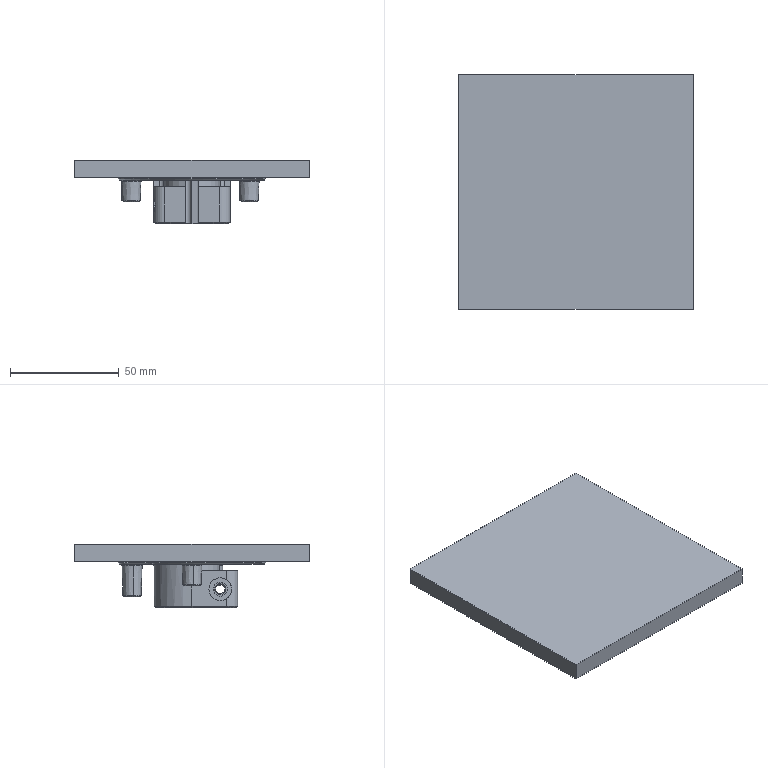NC program | NX | posted with a generic post | part box 108 x 108 x 29 mm
Lines 3489 to 4515 of 23883:
(CAVITY_MILL_COPY_COPY , TOOL : D4)
N6958 T15 M6
N6960 G54
N6962 G17 G0 G90 X0. Y-7.141 S9500 M3
N6964 G43 Z30. H15
N6966 Z-0.385
N6968 G94 G1 X0.5 Y-9.933 F1000.
N6970 G3 X1. Y-9.067 R1.
N6972 G1 X0.541 F1400.
N6974 X0.513 Y-9.112
N6976 X0.51 Y-9.166
N6978 G2 X-0.51 Y-9.166 R0.52
N6980 G1 X-0.513 Y-9.112
N6982 X-0.541 Y-9.067
N6984 X-1.
N6986 Y-20.799
N6988 G3 X-0.51 Y-20.398 R0.5
N6990 G2 X0.51 Y-20.398 R0.52
N6992 G3 X1. Y-20.799 R0.5
N6994 G1 Y-9.067
N6996 G3 X0.5 Y-8.201 R1.
N6998 G1 X0.447 Y-7.069
N7000 G0 X0. Y-7.141 Z-0.769
N7002 G1 X0.5 Y-9.933 F1000.
N7004 G3 X1. Y-9.067 R1.
N7006 G1 X0.541 F1400.
N7008 X0.513 Y-9.112
N7010 X0.51 Y-9.166
N7012 G2 X-0.51 Y-9.166 R0.52
N7014 G1 X-0.513 Y-9.112
N7016 X-0.541 Y-9.067
N7018 X-1.
N7020 Y-20.799
N7022 G3 X-0.51 Y-20.398 R0.5
N7024 G2 X0.51 Y-20.398 R0.52
N7026 G3 X1. Y-20.799 R0.5
N7028 G1 Y-9.067
N7030 G3 X0.5 Y-8.201 R1.
N7032 G1 X0.447 Y-7.069
N7034 G0 X0. Y-7.141 Z-1.154
N7036 G1 X0.5 Y-9.933 F1000.
N7038 G3 X1. Y-9.067 R1.
N7040 G1 X0.541 F1400.
N7042 X0.513 Y-9.112
N7044 X0.51 Y-9.166
N7046 G2 X-0.51 Y-9.166 R0.52
N7048 G1 X-0.513 Y-9.112
N7050 X-0.541 Y-9.067
N7052 X-1.
N7054 Y-20.799
N7056 G3 X-0.51 Y-20.398 R0.5
N7058 G2 X0.51 Y-20.398 R0.52
N7060 G3 X1. Y-20.799 R0.5
N7062 G1 Y-9.067
N7064 G3 X0.5 Y-8.201 R1.
N7066 G1 X0.447 Y-7.069
N7068 G0 X0. Y-7.141 Z-1.538
N7070 G1 X0.5 Y-9.933 F1000.
N7072 G3 X1. Y-9.067 R1.
N7074 G1 X0.541 F1400.
N7076 X0.513 Y-9.112
N7078 X0.51 Y-9.166
N7080 G2 X-0.51 Y-9.166 R0.52
N7082 G1 X-0.513 Y-9.112
N7084 X-0.541 Y-9.067
N7086 X-1.
N7088 Y-20.799
N7090 G3 X-0.51 Y-20.398 R0.5
N7092 G2 X0.51 Y-20.398 R0.52
N7094 G3 X1. Y-20.799 R0.5
N7096 G1 Y-9.067
N7098 G3 X0.5 Y-8.201 R1.
N7100 G1 X0.447 Y-7.069
N7102 G0 X0. Y-7.141 Z-1.923
N7104 G1 X0.5 Y-9.933 F1000.
N7106 G3 X1. Y-9.067 R1.
N7108 G1 X0.541 F1400.
N7110 X0.513 Y-9.112
N7112 X0.51 Y-9.166
N7114 G2 X-0.51 Y-9.166 R0.52
N7116 G1 X-0.513 Y-9.112
N7118 X-0.541 Y-9.067
N7120 X-1.
N7122 Y-20.799
N7124 G3 X-0.51 Y-20.398 R0.5
N7126 G2 X0.51 Y-20.398 R0.52
N7128 G3 X1. Y-20.799 R0.5
N7130 G1 Y-9.067
N7132 G3 X0.5 Y-8.201 R1.
N7134 G1 X0.447 Y-7.069
N7136 G0 X0. Y-7.141 Z-2.308
N7138 G1 X0.5 Y-9.933 F1000.
N7140 G3 X1. Y-9.067 R1.
N7142 G1 X0.541 F1400.
N7144 X0.513 Y-9.112
N7146 X0.51 Y-9.166
N7148 G2 X-0.51 Y-9.166 R0.52
N7150 G1 X-0.513 Y-9.112
N7152 X-0.541 Y-9.067
N7154 X-1.
N7156 Y-20.799
N7158 G3 X-0.51 Y-20.398 R0.5
N7160 G2 X0.51 Y-20.398 R0.52
N7162 G3 X1. Y-20.799 R0.5
N7164 G1 Y-9.067
N7166 G3 X0.5 Y-8.201 R1.
N7168 G1 X0.447 Y-7.069
N7170 G0 X0. Y-7.141 Z-2.692
N7172 G1 X0.5 Y-9.933 F1000.
N7174 G3 X1. Y-9.067 R1.
N7176 G1 X0.541 F1400.
N7178 X0.513 Y-9.112
N7180 X0.51 Y-9.166
N7182 G2 X-0.51 Y-9.166 R0.52
N7184 G1 X-0.513 Y-9.112
N7186 X-0.541 Y-9.067
N7188 X-1.
N7190 Y-20.799
N7192 G3 X-0.51 Y-20.398 R0.5
N7194 G2 X0.51 Y-20.398 R0.52
N7196 G3 X1. Y-20.799 R0.5
N7198 G1 Y-9.067
N7200 G3 X0.5 Y-8.201 R1.
N7202 G1 X0.447 Y-7.069
N7204 G0 X0. Y-7.141 Z-3.077
N7206 G1 X0.5 Y-9.933 F1000.
N7208 G3 X1. Y-9.067 R1.
N7210 G1 X0.541 F1400.
N7212 X0.513 Y-9.112
N7214 X0.51 Y-9.166
N7216 G2 X-0.51 Y-9.166 R0.52
N7218 G1 X-0.513 Y-9.112
N7220 X-0.541 Y-9.067
N7222 X-1.
N7224 Y-20.799
N7226 G3 X-0.51 Y-20.398 R0.5
N7228 G2 X0.51 Y-20.398 R0.52
N7230 G3 X1. Y-20.799 R0.5
N7232 G1 Y-9.067
N7234 G3 X0.5 Y-8.201 R1.
N7236 G1 X0.447 Y-7.069
N7238 G0 X0. Y-7.141 Z-3.462
N7240 G1 X0.5 Y-9.933 F1000.
N7242 G3 X1. Y-9.067 R1.
N7244 G1 X0.541 F1400.
N7246 X0.513 Y-9.112
N7248 X0.51 Y-9.166
N7250 G2 X-0.51 Y-9.166 R0.52
N7252 G1 X-0.513 Y-9.112
N7254 X-0.541 Y-9.067
N7256 X-1.
N7258 Y-20.799
N7260 G3 X-0.51 Y-20.398 R0.5
N7262 G2 X0.51 Y-20.398 R0.52
N7264 G3 X1. Y-20.799 R0.5
N7266 G1 Y-9.067
N7268 G3 X0.5 Y-8.201 R1.
N7270 G1 X0.447 Y-7.069
N7272 G0 X0. Y-7.141 Z-3.846
N7274 G1 X0.5 Y-9.933 F1000.
N7276 G3 X1. Y-9.067 R1.
N7278 G1 X0.541 F1400.
N7280 X0.513 Y-9.112
N7282 X0.51 Y-9.166
N7284 G2 X-0.51 Y-9.166 R0.52
N7286 G1 X-0.513 Y-9.112
N7288 X-0.541 Y-9.067
N7290 X-1.
N7292 Y-20.799
N7294 G3 X-0.51 Y-20.398 R0.5
N7296 G2 X0.51 Y-20.398 R0.52
N7298 G3 X1. Y-20.799 R0.5
N7300 G1 Y-9.067
N7302 G3 X0.5 Y-8.201 R1.
N7304 G1 X0.447 Y-7.069
N7306 G0 X0. Y-7.141 Z-4.231
N7308 G1 X0.5 Y-9.933 F1000.
N7310 G3 X1. Y-9.067 R1.
N7312 G1 X0.541 F1400.
N7314 X0.513 Y-9.112
N7316 X0.51 Y-9.166
N7318 G2 X-0.51 Y-9.166 R0.52
N7320 G1 X-0.513 Y-9.112
N7322 X-0.541 Y-9.067
N7324 X-1.
N7326 Y-20.8
N7328 G3 X-0.51 Y-20.398 R0.5
N7330 G2 X0.51 Y-20.398 R0.52
N7332 G3 X1. Y-20.8 R0.5
N7334 G1 Y-9.067
N7336 G3 X0.5 Y-8.201 R1.
N7338 G1 X0.447 Y-7.069
N7340 G0 X0. Y-7.141 Z-4.615
N7342 G1 X0.5 Y-9.933 F1000.
N7344 G3 X1. Y-9.067 R1.
N7346 G1 X0.541 F1400.
N7348 X0.513 Y-9.112
N7350 X0.51 Y-9.166
N7352 G2 X-0.51 Y-9.166 R0.52
N7354 G1 X-0.513 Y-9.112
N7356 X-0.541 Y-9.067
N7358 X-1.
N7360 Y-20.8
N7362 G3 X-0.51 Y-20.398 R0.5
N7364 G2 X0.51 Y-20.398 R0.52
N7366 G3 X1. Y-20.8 R0.5
N7368 G1 Y-9.067
N7370 G3 X0.5 Y-8.201 R1.
N7372 G1 X0.447 Y-7.069
N7374 G0 X0. Y-7.141 Z-5.
N7376 G1 X0.5 Y-9.933 F1000.
N7378 G3 X1. Y-9.067 R1.
N7380 G1 X0.541 F1400.
N7382 X0.513 Y-9.112
N7384 X0.51 Y-9.166
N7386 G2 X-0.51 Y-9.166 R0.52
N7388 G1 X-0.513 Y-9.112
N7390 X-0.541 Y-9.067
N7392 X-1.
N7394 Y-20.8
N7396 G3 X-0.51 Y-20.398 R0.5
N7398 G2 X0.51 Y-20.398 R0.52
N7400 G3 X1. Y-20.8 R0.5
N7402 G1 Y-9.067
N7404 G3 X0.5 Y-8.201 R1.
N7406 G1 X0.447 Y-7.069
N7408 G0 X0. Y-7.141 Z-5.385
N7410 G1 X0.5 Y-9.933 F1000.
N7412 G3 X1. Y-9.067 R1.
N7414 G1 X0.541 F1400.
N7416 X0.513 Y-9.112
N7418 X0.51 Y-9.166
N7420 G2 X-0.51 Y-9.166 R0.52
N7422 G1 X-0.513 Y-9.112
N7424 X-0.541 Y-9.067
N7426 X-1.
N7428 Y-20.8
N7430 G3 X-0.51 Y-20.398 R0.5
N7432 G2 X0.51 Y-20.398 R0.52
N7434 G3 X1. Y-20.8 R0.5
N7436 G1 Y-9.067
N7438 G3 X0.5 Y-8.201 R1.
N7440 G1 X0.447 Y-7.069
N7442 G0 X0. Y-7.141 Z-5.769
N7444 G1 X0.5 Y-9.933 F1000.
N7446 G3 X1. Y-9.067 R1.
N7448 G1 X0.541 F1400.
N7450 X0.513 Y-9.112
N7452 X0.51 Y-9.166
N7454 G2 X-0.51 Y-9.166 R0.52
N7456 G1 X-0.513 Y-9.112
N7458 X-0.541 Y-9.067
N7460 X-1.
N7462 Y-20.8
N7464 G3 X-0.51 Y-20.398 R0.5
N7466 G2 X0.51 Y-20.398 R0.52
N7468 G3 X1. Y-20.8 R0.5
N7470 G1 Y-9.067
N7472 G3 X0.5 Y-8.201 R1.
N7474 G1 X0.447 Y-7.069
N7476 G0 X0. Y-7.141 Z-6.154
N7478 G1 X0.5 Y-9.933 F1000.
N7480 G3 X1. Y-9.067 R1.
N7482 G1 X0.542 F1400.
N7484 X0.514 Y-9.114
N7486 X0.51 Y-9.169
N7488 G2 X-0.51 Y-9.169 R0.52
N7490 G1 X-0.514 Y-9.114
N7492 X-0.542 Y-9.067
N7494 X-1.
N7496 Y-20.8
N7498 G3 X-0.51 Y-20.398 R0.5
N7500 G2 X0.51 Y-20.398 R0.52
N7502 G3 X1. Y-20.8 R0.5
N7504 G1 Y-9.067
N7506 G3 X0.5 Y-8.201 R1.
N7508 G1 X0.445 Y-7.069
N7510 G0 X0. Y-7.141 Z-6.538
N7512 G1 X0.5 Y-9.933 F1000.
N7514 G3 X1. Y-9.067 R1.
N7516 G1 X0.542 F1400.
N7518 X0.514 Y-9.114
N7520 X0.51 Y-9.169
N7522 G2 X-0.51 Y-9.169 R0.52
N7524 G1 X-0.514 Y-9.114
N7526 X-0.542 Y-9.067
N7528 X-1.
N7530 Y-20.8
N7532 G3 X-0.51 Y-20.398 R0.5
N7534 G2 X0.51 Y-20.398 R0.52
N7536 G3 X1. Y-20.8 R0.5
N7538 G1 Y-9.067
N7540 G3 X0.5 Y-8.201 R1.
N7542 G1 X0.445 Y-7.069
N7544 G0 X0. Y-7.141 Z-6.923
N7546 G1 X0.5 Y-9.933 F1000.
N7548 G3 X1. Y-9.067 R1.
N7550 G1 X0.542 F1400.
N7552 X0.514 Y-9.114
N7554 X0.51 Y-9.169
N7556 G2 X-0.51 Y-9.169 R0.52
N7558 G1 X-0.514 Y-9.114
N7560 X-0.542 Y-9.067
N7562 X-1.
N7564 Y-20.8
N7566 G3 X-0.51 Y-20.398 R0.5
N7568 G2 X0.51 Y-20.398 R0.52
N7570 G3 X1. Y-20.8 R0.5
N7572 G1 Y-9.067
N7574 G3 X0.5 Y-8.201 R1.
N7576 G1 X0.445 Y-7.069
N7578 G0 X0. Y-7.141 Z-7.308
N7580 G1 X0.5 Y-9.933 F1000.
N7582 G3 X1. Y-9.067 R1.
N7584 G1 X0.541 F1400.
N7586 X0.513 Y-9.112
N7588 X0.51 Y-9.166
N7590 G2 X-0.51 Y-9.166 R0.52
N7592 G1 X-0.513 Y-9.112
N7594 X-0.541 Y-9.067
N7596 X-1.
N7598 Y-20.8
N7600 G3 X-0.51 Y-20.398 R0.5
N7602 G2 X0.51 Y-20.398 R0.52
N7604 G3 X1. Y-20.8 R0.5
N7606 G1 Y-9.067
N7608 G3 X0.5 Y-8.201 R1.
N7610 G1 X0.447 Y-7.069
N7612 G0 X0. Y-7.141 Z-7.692
N7614 G1 X0.5 Y-9.933 F1000.
N7616 G3 X1. Y-9.067 R1.
N7618 G1 X0.541 F1400.
N7620 X0.513 Y-9.112
N7622 X0.51 Y-9.166
N7624 G2 X-0.51 Y-9.166 R0.52
N7626 G1 X-0.513 Y-9.112
N7628 X-0.541 Y-9.067
N7630 X-1.
N7632 Y-20.8
N7634 G3 X-0.51 Y-20.398 R0.5
N7636 G2 X0.51 Y-20.398 R0.52
N7638 G3 X1. Y-20.8 R0.5
N7640 G1 Y-9.067
N7642 G3 X0.5 Y-8.201 R1.
N7644 G1 X0.447 Y-7.069
N7646 G0 X0. Y-7.141 Z-8.077
N7648 G1 X0.5 Y-9.933 F1000.
N7650 G3 X1. Y-9.067 R1.
N7652 G1 X0.541 F1400.
N7654 X0.513 Y-9.112
N7656 X0.51 Y-9.166
N7658 G2 X-0.51 Y-9.166 R0.52
N7660 G1 X-0.513 Y-9.112
N7662 X-0.541 Y-9.067
N7664 X-1.
N7666 Y-20.8
N7668 G3 X-0.51 Y-20.398 R0.5
N7670 G2 X0.51 Y-20.398 R0.52
N7672 G3 X1. Y-20.8 R0.5
N7674 G1 Y-9.067
N7676 G3 X0.5 Y-8.201 R1.
N7678 G1 X0.447 Y-7.069
N7680 G0 X0. Y-7.141 Z-8.462
N7682 G1 X0.5 Y-9.933 F1000.
N7684 G3 X1. Y-9.067 R1.
N7686 G1 X0.541 F1400.
N7688 X0.513 Y-9.112
N7690 X0.51 Y-9.166
N7692 G2 X-0.51 Y-9.166 R0.52
N7694 G1 X-0.513 Y-9.112
N7696 X-0.541 Y-9.067
N7698 X-1.
N7700 Y-20.8
N7702 G3 X-0.51 Y-20.399 R0.5
N7704 G2 X0.51 Y-20.399 R0.52
N7706 G3 X1. Y-20.8 R0.5
N7708 G1 Y-9.067
N7710 G3 X0.5 Y-8.201 R1.
N7712 G1 X0.447 Y-7.069
N7714 G0 X0. Y-7.141 Z-8.846
N7716 G1 X0.5 Y-9.933 F1000.
N7718 G3 X1. Y-9.067 R1.
N7720 G1 X0.541 F1400.
N7722 X0.513 Y-9.112
N7724 X0.51 Y-9.166
N7726 G2 X-0.51 Y-9.166 R0.52
N7728 G1 X-0.513 Y-9.112
N7730 X-0.541 Y-9.067
N7732 X-1.
N7734 Y-20.8
N7736 G3 X-0.51 Y-20.399 R0.5
N7738 G2 X0.51 Y-20.399 R0.52
N7740 G3 X1. Y-20.8 R0.5
N7742 G1 Y-9.067
N7744 G3 X0.5 Y-8.201 R1.
N7746 G1 X0.447 Y-7.069
N7748 G0 X0. Y-7.141 Z-9.231
N7750 G1 X0.5 Y-9.933 F1000.
N7752 G3 X1. Y-9.067 R1.
N7754 G1 X0.541 F1400.
N7756 X0.513 Y-9.112
N7758 X0.51 Y-9.166
N7760 G2 X-0.51 Y-9.166 R0.52
N7762 G1 X-0.513 Y-9.112
N7764 X-0.541 Y-9.067
N7766 X-1.
N7768 Y-20.8
N7770 G3 X-0.51 Y-20.399 R0.5
N7772 G2 X0.51 Y-20.399 R0.52
N7774 G3 X1. Y-20.8 R0.5
N7776 G1 Y-9.067
N7778 G3 X0.5 Y-8.201 R1.
N7780 G1 X0.447 Y-7.069
N7782 G0 X0. Y-7.141 Z-9.615
N7784 G1 X0.5 Y-9.933 F1000.
N7786 G3 X1. Y-9.067 R1.
N7788 G1 X0.541 F1400.
N7790 X0.513 Y-9.112
N7792 X0.51 Y-9.166
N7794 G2 X-0.51 Y-9.166 R0.52
N7796 G1 X-0.513 Y-9.112
N7798 X-0.541 Y-9.067
N7800 X-1.
N7802 Y-20.8
N7804 G3 X-0.51 Y-20.399 R0.5
N7806 G2 X0.51 Y-20.399 R0.52
N7808 G3 X1. Y-20.8 R0.5
N7810 G1 Y-9.067
N7812 G3 X0.5 Y-8.201 R1.
N7814 G1 X0.447 Y-7.069
N7816 G0 X0. Y-7.141 Z-10.
N7818 G1 X0.5 Y-9.933 F1000.
N7820 G3 X1. Y-9.067 R1.
N7822 G1 X0.542 F1400.
N7824 X0.514 Y-9.114
N7826 X0.51 Y-9.169
N7828 G2 X-0.51 Y-9.169 R0.52
N7830 G1 X-0.514 Y-9.114
N7832 X-0.542 Y-9.067
N7834 X-1.
N7836 Y-20.8
N7838 G3 X-0.51 Y-20.399 R0.5
N7840 G2 X0.51 Y-20.399 R0.52
N7842 G3 X1. Y-20.8 R0.5
N7844 G1 Y-9.067
N7846 G3 X0.5 Y-8.201 R1.
N7848 G1 X0.445 Y-7.069
N7850 G0 X0. Y-7.141 Z-10.4
N7852 G1 X0.5 Y-9.933 F1000.
N7854 G3 X1. Y-9.067 R1.
N7856 G1 X0.542 F1400.
N7858 X0.514 Y-9.114
N7860 X0.51 Y-9.169
N7862 G2 X-0.51 Y-9.169 R0.52
N7864 G1 X-0.514 Y-9.114
N7866 X-0.542 Y-9.067
N7868 X-1.
N7870 Y-20.8
N7872 G3 X-0.51 Y-20.399 R0.5
N7874 G2 X0.51 Y-20.399 R0.52
N7876 G3 X1. Y-20.8 R0.5
N7878 G1 Y-9.067
N7880 G3 X0.5 Y-8.201 R1.
N7882 G1 X0.445 Y-7.069
N7884 G0 X0. Y-7.141 Z-10.8
N7886 G1 X0.5 Y-9.933 F1000.
N7888 G3 X1. Y-9.067 R1.
N7890 G1 X0.542 F1400.
N7892 X0.514 Y-9.114
N7894 X0.51 Y-9.169
N7896 G2 X-0.51 Y-9.169 R0.52
N7898 G1 X-0.514 Y-9.114
N7900 X-0.542 Y-9.067
N7902 X-1.
N7904 Y-20.8
N7906 G3 X-0.51 Y-20.399 R0.5
N7908 G2 X0.51 Y-20.399 R0.52
N7910 G3 X1. Y-20.8 R0.5
N7912 G1 Y-9.067
N7914 G3 X0.5 Y-8.201 R1.
N7916 G1 X0.445 Y-7.069
N7918 G0 X0. Y-7.141 Z-11.2
N7920 G1 X0.5 Y-9.933 F1000.
N7922 G3 X1. Y-9.067 R1.
N7924 G1 X0.542 F1400.
N7926 X0.514 Y-9.114
N7928 X0.51 Y-9.169
N7930 G2 X-0.51 Y-9.169 R0.52
N7932 G1 X-0.514 Y-9.114
N7934 X-0.542 Y-9.067
N7936 X-1.
N7938 Y-20.8
N7940 G3 X-0.51 Y-20.399 R0.5
N7942 G2 X0.51 Y-20.399 R0.52
N7944 G3 X1. Y-20.8 R0.5
N7946 G1 Y-9.067
N7948 G3 X0.5 Y-8.201 R1.
N7950 G1 X0.445 Y-7.069
N7952 G0 X0. Y-7.141 Z-11.6
N7954 G1 X0.5 Y-9.933 F1000.
N7956 G3 X1. Y-9.067 R1.
N7958 G1 X0.542 F1400.
N7960 X0.514 Y-9.114
N7962 X0.51 Y-9.169
N7964 G2 X-0.51 Y-9.169 R0.52
N7966 G1 X-0.514 Y-9.114
N7968 X-0.542 Y-9.067
N7970 X-1.
N7972 Y-20.8
N7974 G3 X-0.51 Y-20.399 R0.5
N7976 G2 X0.51 Y-20.399 R0.52
N7978 G3 X1. Y-20.8 R0.5
N7980 G1 Y-9.067
N7982 G3 X0.5 Y-8.201 R1.
N7984 G1 X0.445 Y-7.069
N7986 G0 X0. Y-7.141 Z-12.
N7988 G1 X0.5 Y-9.933 F1000.
N7990 G3 X1. Y-9.067 R1.
N7992 G1 X0.542 F1400.
N7994 X0.514 Y-9.114
N7996 X0.51 Y-9.168
N7998 G2 X-0.51 Y-9.168 R0.52
N8000 G1 X-0.514 Y-9.114
N8002 X-0.542 Y-9.067
N8004 X-1.
N8006 Y-20.8
N8008 G3 X-0.51 Y-20.399 R0.5
N8010 G2 X0.51 Y-20.399 R0.52
N8012 G3 X1. Y-20.8 R0.5
N8014 G1 Y-9.067
N8016 G3 X0.5 Y-8.201 R1.
N8018 G1 X0.445 Y-7.069
N8020 G0 X0. Y-7.141 Z-12.4
N8022 G1 X0.5 Y-9.933 F1000.
N8024 G3 X1. Y-9.067 R1.
N8026 G1 X0.542 F1400.
N8028 X0.514 Y-9.114
N8030 X0.51 Y-9.168
N8032 G2 X-0.51 Y-9.168 R0.52
N8034 G1 X-0.514 Y-9.114
N8036 X-0.542 Y-9.067
N8038 X-1.
N8040 Y-20.8
N8042 G3 X-0.51 Y-20.399 R0.5
N8044 G2 X0.51 Y-20.399 R0.52
N8046 G3 X1. Y-20.8 R0.5
N8048 G1 Y-9.067
N8050 G3 X0.5 Y-8.201 R1.
N8052 G1 X0.445 Y-7.069
N8054 G0 X0. Y-7.141 Z-12.8
N8056 G1 X0.5 Y-9.933 F1000.
N8058 G3 X1. Y-9.067 R1.
N8060 G1 X0.542 F1400.
N8062 X0.514 Y-9.114
N8064 X0.51 Y-9.168
N8066 G2 X-0.51 Y-9.168 R0.52
N8068 G1 X-0.514 Y-9.114
N8070 X-0.542 Y-9.067
N8072 X-1.
N8074 Y-20.801
N8076 G3 X-0.51 Y-20.399 R0.5
N8078 G2 X0.51 Y-20.399 R0.52
N8080 G3 X1. Y-20.801 R0.5
N8082 G1 Y-9.067
N8084 G3 X0.5 Y-8.201 R1.
N8086 G1 X0.445 Y-7.069
N8088 G0 X0. Y-7.141 Z-13.2
N8090 G1 X0.5 Y-9.933 F1000.
N8092 G3 X1. Y-9.067 R1.
N8094 G1 X0.542 F1400.
N8096 X0.514 Y-9.114
N8098 X0.51 Y-9.168
N8100 G2 X-0.51 Y-9.168 R0.52
N8102 G1 X-0.514 Y-9.114
N8104 X-0.542 Y-9.067
N8106 X-1.
N8108 Y-20.801
N8110 G3 X-0.51 Y-20.399 R0.5
N8112 G2 X0.51 Y-20.399 R0.52
N8114 G3 X1. Y-20.801 R0.5
N8116 G1 Y-9.067
N8118 G3 X0.5 Y-8.201 R1.
N8120 G1 X0.445 Y-7.069
N8122 G0 X0. Y-7.141 Z-13.6
N8124 G1 X0.5 Y-9.933 F1000.
N8126 G3 X1. Y-9.067 R1.
N8128 G1 X0.542 F1400.
N8130 X0.514 Y-9.114
N8132 X0.51 Y-9.168
N8134 G2 X-0.51 Y-9.168 R0.52
N8136 G1 X-0.514 Y-9.114
N8138 X-0.542 Y-9.067
N8140 X-1.
N8142 Y-20.801
N8144 G3 X-0.51 Y-20.399 R0.5
N8146 G2 X0.51 Y-20.399 R0.52
N8148 G3 X1. Y-20.801 R0.5
N8150 G1 Y-9.067
N8152 G3 X0.5 Y-8.201 R1.
N8154 G1 X0.445 Y-7.069
N8156 G0 X0. Y-7.141 Z-14.
N8158 G1 X0.5 Y-9.933 F1000.
N8160 G3 X1. Y-9.067 R1.
N8162 G1 X0.542 F1400.
N8164 X0.514 Y-9.113
N8166 X0.51 Y-9.168
N8168 G2 X-0.51 Y-9.168 R0.52
N8170 G1 X-0.514 Y-9.113
N8172 X-0.542 Y-9.067
N8174 X-1.
N8176 Y-20.801
N8178 G3 X-0.51 Y-20.399 R0.5
N8180 G2 X0.51 Y-20.399 R0.52
N8182 G3 X1. Y-20.801 R0.5
N8184 G1 Y-9.067
N8186 G3 X0.5 Y-8.201 R1.
N8188 G1 X0.445 Y-7.069
N8190 G0 X0. Y-7.141 Z-14.4
N8192 G1 X0.5 Y-9.933 F1000.
N8194 G3 X1. Y-9.067 R1.
N8196 G1 X0.542 F1400.
N8198 X0.514 Y-9.113
N8200 X0.51 Y-9.168
N8202 G2 X-0.51 Y-9.168 R0.52
N8204 G1 X-0.514 Y-9.113
N8206 X-0.542 Y-9.067
N8208 X-1.
N8210 Y-20.801
N8212 G3 X-0.51 Y-20.399 R0.5
N8214 G2 X0.51 Y-20.399 R0.52
N8216 G3 X1. Y-20.801 R0.5
N8218 G1 Y-9.067
N8220 G3 X0.5 Y-8.201 R1.
N8222 G1 X0.445 Y-7.069
N8224 G0 X0. Y-7.141 Z-14.8
N8226 G1 X0.5 Y-9.933 F1000.
N8228 G3 X1. Y-9.067 R1.
N8230 G1 X0.542 F1400.
N8232 X0.514 Y-9.113
N8234 X0.51 Y-9.168
N8236 G2 X-0.51 Y-9.168 R0.52
N8238 G1 X-0.514 Y-9.113
N8240 X-0.542 Y-9.067
N8242 X-1.
N8244 Y-20.801
N8246 G3 X-0.51 Y-20.399 R0.5
N8248 G2 X0.51 Y-20.399 R0.52
N8250 G3 X1. Y-20.801 R0.5
N8252 G1 Y-9.067
N8254 G3 X0.5 Y-8.201 R1.
N8256 G1 X0.445 Y-7.069
N8258 G0 X0. Y-7.141 Z-15.2
N8260 G1 X0.5 Y-9.933 F1000.
N8262 G3 X1. Y-9.067 R1.
N8264 G1 X0.542 F1400.
N8266 X0.514 Y-9.113
N8268 X0.51 Y-9.168
N8270 G2 X-0.51 Y-9.168 R0.52
N8272 G1 X-0.514 Y-9.113
N8274 X-0.542 Y-9.067
N8276 X-1.
N8278 Y-20.801
N8280 G3 X-0.51 Y-20.399 R0.5
N8282 G2 X0.51 Y-20.399 R0.52
N8284 G3 X1. Y-20.801 R0.5
N8286 G1 Y-9.067
N8288 G3 X0.5 Y-8.201 R1.
N8290 G1 X0.445 Y-7.069
N8292 G0 X0. Y-7.141 Z-15.6
N8294 G1 X0.5 Y-9.933 F1000.
N8296 G3 X1. Y-9.067 R1.
N8298 G1 X0.542 F1400.
N8300 X0.514 Y-9.113
N8302 X0.51 Y-9.168
N8304 G2 X-0.51 Y-9.168 R0.52
N8306 G1 X-0.514 Y-9.113
N8308 X-0.542 Y-9.067
N8310 X-1.
N8312 Y-20.801
N8314 G3 X-0.51 Y-20.399 R0.5
N8316 G2 X0.51 Y-20.399 R0.52
N8318 G3 X1. Y-20.801 R0.5
N8320 G1 Y-9.067
N8322 G3 X0.5 Y-8.201 R1.
N8324 G1 X0.446 Y-7.069
N8326 G0 X0. Y-7.141 Z-16.
N8328 G1 X0.5 Y-9.933 F1000.
N8330 G3 X1. Y-9.067 R1.
N8332 G1 X0.542 F1400.
N8334 X0.513 Y-9.113
N8336 X0.51 Y-9.168
N8338 G2 X-0.51 Y-9.168 R0.52
N8340 G1 X-0.513 Y-9.113
N8342 X-0.542 Y-9.067
N8344 X-1.
N8346 Y-20.801
N8348 G3 X-0.51 Y-20.399 R0.5
N8350 G2 X0.51 Y-20.399 R0.52
N8352 G3 X1. Y-20.801 R0.5
N8354 G1 Y-9.067
N8356 G3 X0.5 Y-8.201 R1.
N8358 G1 X0.446 Y-7.069
N8360 G0 X0. Y-7.141 Z-16.4
N8362 G1 X0.5 Y-9.933 F1000.
N8364 G3 X1. Y-9.067 R1.
N8366 G1 X0.542 F1400.
N8368 X0.513 Y-9.113
N8370 X0.51 Y-9.168
N8372 G2 X-0.51 Y-9.168 R0.52
N8374 G1 X-0.513 Y-9.113
N8376 X-0.542 Y-9.067
N8378 X-1.
N8380 Y-20.801
N8382 G3 X-0.51 Y-20.399 R0.5
N8384 G2 X0.51 Y-20.399 R0.52
N8386 G3 X1. Y-20.801 R0.5
N8388 G1 Y-9.067
N8390 G3 X0.5 Y-8.201 R1.
N8392 G1 X0.446 Y-7.069
N8394 G0 X0. Y-7.141 Z-16.8
N8396 G1 X0.5 Y-9.933 F1000.
N8398 G3 X1. Y-9.067 R1.
N8400 G1 X0.542 F1400.
N8402 X0.513 Y-9.113
N8404 X0.51 Y-9.168
N8406 G2 X-0.51 Y-9.168 R0.52
N8408 G1 X-0.513 Y-9.113
N8410 X-0.542 Y-9.067
N8412 X-1.
N8414 Y-20.801
N8416 G3 X-0.51 Y-20.4 R0.5
N8418 G2 X0.51 Y-20.4 R0.52
N8420 G3 X1. Y-20.801 R0.5
N8422 G1 Y-9.067
N8424 G3 X0.5 Y-8.201 R1.
N8426 G1 X0.446 Y-7.069
N8428 G0 X0. Y-7.141 Z-17.2
N8430 G1 X0.5 Y-9.933 F1000.
N8432 G3 X1. Y-9.067 R1.
N8434 G1 X0.542 F1400.
N8436 X0.514 Y-9.114
N8438 X0.51 Y-9.168
N8440 G2 X-0.51 Y-9.168 R0.52
N8442 G1 X-0.514 Y-9.114
N8444 X-0.542 Y-9.067
N8446 X-1.
N8448 Y-21.
N8450 G2 X-1.063 Y-21.499 R2.
N8452 G3 X-0.515 Y-21.124 R0.5
N8454 G2 X-0.359 Y-20.863 R0.521
N8456 X0.514 Y-21.108 R0.52
N8458 G3 X1.06 Y-21.486 R0.5
N8460 G2 X1. Y-21. R2.
N8462 G1 Y-9.067
N8464 G3 X0.5 Y-8.201 R1.
N8466 G1 X0.445 Y-7.069
N8468 G0 X0. Y-7.141 Z-17.6
N8470 G1 X0.5 Y-9.933 F1000.
N8472 G3 X1. Y-9.067 R1.
N8474 G1 X0.542 F1400.
N8476 X0.514 Y-9.113
N8478 X0.51 Y-9.168
N8480 G2 X-0.51 Y-9.168 R0.52
N8482 G1 X-0.514 Y-9.113
N8484 X-0.542 Y-9.067
N8486 X-1.
N8488 Y-21.
N8490 G2 X-1.022 Y-21.299 R2.
N8492 G3 X-0.51 Y-20.898 R0.5
N8494 G2 X0.51 Y-20.898 R0.52
N8496 G3 X1.022 Y-21.299 R0.5
N8498 G2 X1. Y-21. R2.
N8500 G1 Y-9.067
N8502 G3 X0.5 Y-8.201 R1.
N8504 G1 X0.445 Y-7.069
N8506 G0 X0. Y-7.141 Z-18.
N8508 G1 X0.5 Y-9.933 F1000.
N8510 G3 X1. Y-9.067 R1.
N8512 G1 X0.542 F1400.
N8514 X0.514 Y-9.113
N8516 X0.51 Y-9.168
N8518 G2 X-0.51 Y-9.168 R0.52
N8520 G1 X-0.514 Y-9.113
N8522 X-0.542 Y-9.067
N8524 X-1.
N8526 Y-21.
N8528 G2 X-1.063 Y-21.499 R2.
N8530 G3 X-0.515 Y-21.124 R0.5
N8532 G2 X-0.36 Y-20.864 R0.521
N8534 X0.514 Y-21.108 R0.52
N8536 G3 X1.06 Y-21.486 R0.5
N8538 G2 X1. Y-21. R2.
N8540 G1 Y-9.067
N8542 G3 X0.5 Y-8.201 R1.
N8544 G1 X0.445 Y-7.069
N8546 G0 X0. Y-7.141 Z-18.4
N8548 G1 X0.5 Y-9.933 F1000.
N8550 G3 X1. Y-9.067 R1.
N8552 G1 X0.542 F1400.
N8554 X0.514 Y-9.113
N8556 X0.51 Y-9.168
N8558 G2 X-0.51 Y-9.168 R0.52
N8560 G1 X-0.514 Y-9.113
N8562 X-0.542 Y-9.067
N8564 X-1.
N8566 Y-21.
N8568 G2 X-1.022 Y-21.299 R2.
N8570 G3 X-0.51 Y-20.898 R0.5
N8572 G2 X0.51 Y-20.898 R0.52
N8574 G3 X1.022 Y-21.299 R0.5
N8576 G2 X1. Y-21. R2.
N8578 G1 Y-9.067
N8580 G3 X0.5 Y-8.201 R1.
N8582 G1 X0.445 Y-7.069
N8584 G0 X0. Y-7.141 Z-18.8
N8586 G1 X0.5 Y-9.933 F1000.
N8588 G3 X1. Y-9.067 R1.
N8590 G1 X0.542 F1400.
N8592 X0.514 Y-9.113
N8594 X0.51 Y-9.168
N8596 G2 X-0.51 Y-9.168 R0.52
N8598 G1 X-0.514 Y-9.113
N8600 X-0.542 Y-9.067
N8602 X-1.
N8604 Y-21.
N8606 G2 X-1.063 Y-21.499 R2.
N8608 G3 X-0.515 Y-21.124 R0.5
N8610 G2 X-0.36 Y-20.864 R0.521
N8612 X0.514 Y-21.108 R0.52
N8614 G3 X1.06 Y-21.486 R0.5
N8616 G2 X1. Y-21. R2.
N8618 G1 Y-9.067
N8620 G3 X0.5 Y-8.201 R1.
N8622 G1 X0.445 Y-7.069
N8624 G0 X0. Y-7.141 Z-19.2
N8626 G1 X0.5 Y-9.933 F1000.
N8628 G3 X1. Y-9.067 R1.
N8630 G1 X0.542 F1400.
N8632 X0.514 Y-9.113
N8634 X0.51 Y-9.168
N8636 G2 X-0.51 Y-9.168 R0.52
N8638 G1 X-0.514 Y-9.113
N8640 X-0.542 Y-9.067
N8642 X-1.
N8644 Y-21.
N8646 G2 X-1.022 Y-21.299 R2.
N8648 G3 X-0.51 Y-20.898 R0.5
N8650 G2 X0.51 Y-20.898 R0.52
N8652 G3 X1.022 Y-21.299 R0.5
N8654 G2 X1. Y-21. R2.
N8656 G1 Y-9.067
N8658 G3 X0.5 Y-8.201 R1.
N8660 G1 X0.445 Y-7.069
N8662 G0 X0. Y-7.141 Z-19.6
N8664 G1 X0.5 Y-9.933 F1000.
N8666 G3 X1. Y-9.067 R1.
N8668 G1 X0.542 F1400.
N8670 X0.514 Y-9.113
N8672 X0.51 Y-9.168
N8674 G2 X-0.51 Y-9.168 R0.52
N8676 G1 X-0.514 Y-9.113
N8678 X-0.542 Y-9.067
N8680 X-1.
N8682 Y-21.
N8684 G2 X-1.063 Y-21.499 R2.
N8686 G3 X-0.515 Y-21.124 R0.5
N8688 G2 X-0.361 Y-20.865 R0.521
N8690 X0.514 Y-21.108 R0.52
N8692 G3 X1.06 Y-21.486 R0.5
N8694 G2 X1. Y-21. R2.
N8696 G1 Y-9.067
N8698 G3 X0.5 Y-8.201 R1.
N8700 G1 X0.445 Y-7.069
N8702 G0 X0. Y-7.141 Z-20.
N8704 G1 X0.5 Y-9.933 F1000.
N8706 G3 X1. Y-9.067 R1.
N8708 G1 X0.542 F1400.
N8710 X0.514 Y-9.113
N8712 X0.51 Y-9.168
N8714 G2 X-0.51 Y-9.168 R0.52
N8716 G1 X-0.514 Y-9.113
N8718 X-0.542 Y-9.067
N8720 X-1.
N8722 Y-21.
N8724 G2 X-1.023 Y-21.299 R2.
N8726 G3 X-0.51 Y-20.898 R0.5
N8728 G2 X0.51 Y-20.898 R0.52
N8730 G3 X1.023 Y-21.299 R0.5
N8732 G2 X1. Y-21. R2.
N8734 G1 Y-9.067
N8736 G3 X0.5 Y-8.201 R1.
N8738 G1 X0.445 Y-7.069
N8740 G0 X0. Y-7.141 Z-20.385
N8742 G1 X0.5 Y-9.933 F1000.
N8744 G3 X1. Y-9.067 R1.
N8746 G1 X0.542 F1400.
N8748 X0.514 Y-9.113
N8750 X0.51 Y-9.168
N8752 G2 X-0.51 Y-9.168 R0.52
N8754 G1 X-0.514 Y-9.113
N8756 X-0.542 Y-9.067
N8758 X-1.
N8760 Y-21.
N8762 X1.
N8764 Y-9.067
N8766 G3 X0.5 Y-8.201 R1.
N8768 G1 X0.445 Y-7.069
N8770 G0 X0. Y-7.141 Z-20.769
N8772 G1 X0.5 Y-9.933 F1000.
N8774 G3 X1. Y-9.067 R1.
N8776 G1 X0.542 F1400.
N8778 X0.514 Y-9.113
N8780 X0.51 Y-9.168
N8782 G2 X-0.51 Y-9.168 R0.52
N8784 G1 X-0.514 Y-9.113
N8786 X-0.542 Y-9.067
N8788 X-1.
N8790 Y-21.
N8792 X1.
N8794 Y-9.067
N8796 G3 X0.5 Y-8.201 R1.
N8798 G1 X0.446 Y-7.069
N8800 G0 X0. Y-7.141 Z-21.154
N8802 G1 X0.5 Y-9.933 F1000.
N8804 G3 X1. Y-9.067 R1.
N8806 G1 X0.542 F1400.
N8808 X0.514 Y-9.113
N8810 X0.51 Y-9.168
N8812 G2 X-0.51 Y-9.168 R0.52
N8814 G1 X-0.514 Y-9.113
N8816 X-0.542 Y-9.067
N8818 X-1.
N8820 Y-21.
N8822 X1.
N8824 Y-9.067
N8826 G3 X0.5 Y-8.201 R1.
N8828 G1 X0.446 Y-7.069
N8830 G0 X0. Y-7.141 Z-21.538
N8832 G1 X0.5 Y-9.933 F1000.
N8834 G3 X1. Y-9.067 R1.
N8836 G1 X0.542 F1400.
N8838 X0.514 Y-9.113
N8840 X0.51 Y-9.168
N8842 G2 X-0.51 Y-9.168 R0.52
N8844 G1 X-0.514 Y-9.113
N8846 X-0.542 Y-9.067
N8848 X-1.
N8850 Y-21.
N8852 X1.
N8854 Y-9.067
N8856 G3 X0.5 Y-8.201 R1.
N8858 G1 X0.446 Y-7.069
N8860 G0 X0. Y-7.141 Z-21.923
N8862 G1 X0.5 Y-9.933 F1000.
N8864 G3 X1. Y-9.067 R1.
N8866 G1 X0.542 F1400.
N8868 X0.514 Y-9.113
N8870 X0.51 Y-9.168
N8872 G2 X-0.51 Y-9.168 R0.52
N8874 G1 X-0.514 Y-9.113
N8876 X-0.542 Y-9.067
N8878 X-1.
N8880 Y-21.
N8882 X1.
N8884 Y-9.067
N8886 G3 X0.5 Y-8.201 R1.
N8888 G1 X0.446 Y-7.069
N8890 G0 X0. Y-7.141 Z-22.308
N8892 G1 X0.5 Y-9.933 F1000.
N8894 G3 X1. Y-9.067 R1.
N8896 G1 X0.542 F1400.
N8898 X0.513 Y-9.113
N8900 X0.51 Y-9.168
N8902 G2 X-0.51 Y-9.168 R0.52
N8904 G1 X-0.513 Y-9.113
N8906 X-0.542 Y-9.067
N8908 X-1.
N8910 Y-21.
N8912 X1.
N8914 Y-9.067
N8916 G3 X0.5 Y-8.201 R1.
N8918 G1 X0.446 Y-7.069
N8920 G0 X0. Y-7.141 Z-22.692
N8922 G1 X0.5 Y-9.933 F1000.
N8924 G3 X1. Y-9.067 R1.
N8926 G1 X0.542 F1400.
N8928 X0.513 Y-9.113
N8930 X0.51 Y-9.168
N8932 G2 X-0.51 Y-9.168 R0.52
N8934 G1 X-0.513 Y-9.113
N8936 X-0.542 Y-9.067
N8938 X-1.
N8940 Y-21.
N8942 X1.
N8944 Y-9.067
N8946 G3 X0.5 Y-8.201 R1.
N8948 G1 X0.446 Y-7.069
N8950 G0 X0. Y-7.141 Z-23.077
N8952 G1 X0.5 Y-9.933 F1000.
N8954 G3 X1. Y-9.067 R1.
N8956 G1 X0.542 F1400.
N8958 X0.513 Y-9.113
N8960 X0.51 Y-9.168
N8962 G2 X-0.51 Y-9.168 R0.52
N8964 G1 X-0.513 Y-9.113
N8966 X-0.542 Y-9.067
N8968 X-1.
N8970 Y-21.
N8972 X1.
N8974 Y-9.067
N8976 G3 X0.5 Y-8.201 R1.
N8978 G1 X0.446 Y-7.069
N8980 G0 X0. Y-7.141 Z-23.462
N8982 G1 X0.5 Y-9.933 F1000.
N8984 G3 X1. Y-9.067 R1.
N8986 G1 X0.542 F1400.
N8988 X0.513 Y-9.113
N8990 X0.51 Y-9.168
N8992 G2 X-0.51 Y-9.168 R0.52
N8994 G1 X-0.513 Y-9.113
N8996 X-0.542 Y-9.067
N8998 X-1.
N9000 Y-21.
N9002 X1.
N9004 Y-9.067